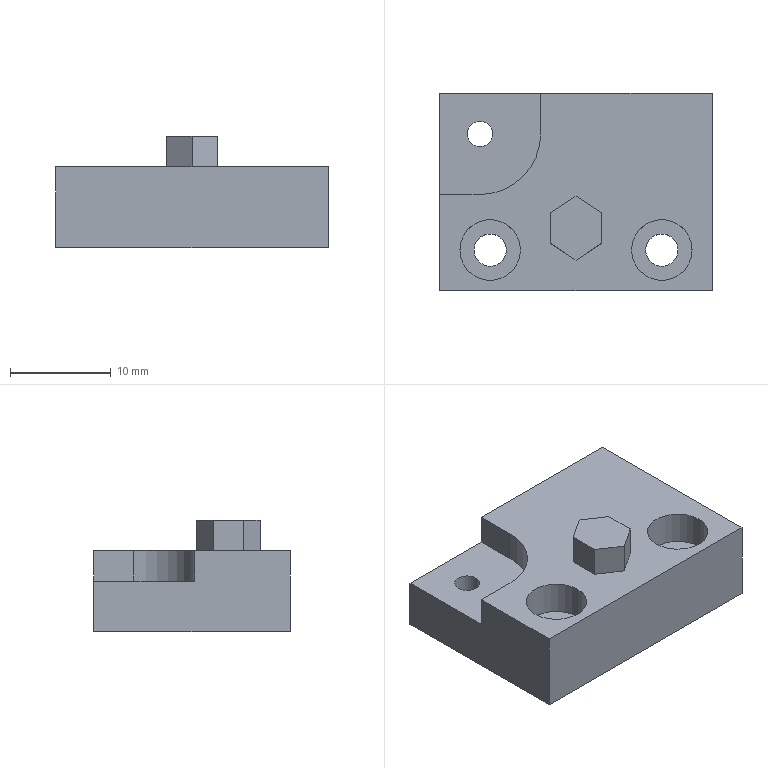Part | NX | 1 solid | 33 faces | box 27 x 19.5 x 11 mm | volume 3538 mm3 | plane 18 | cylinder 13 | cone 2 | commonest cylinder face diameters 3.2 x4 6 x4 2.5 x2 4.2 x2 12 x1
STEP:
#1=CARTESIAN_POINT('',(27.,0.,0.));
#2=VERTEX_POINT('',#1);
#3=CARTESIAN_POINT('',(0.,0.,0.));
#4=VERTEX_POINT('',#3);
#5=CARTESIAN_POINT('',(27.,0.,0.));
#6=DIRECTION('',(-1.,0.,0.));
#7=VECTOR('',#6,1000.);
#8=LINE('',#5,#7);
#9=EDGE_CURVE('',#2,#4,#8,.T.);
#10=ORIENTED_EDGE('',*,*,#9,.T.);
#11=CARTESIAN_POINT('',(0.,19.5,0.));
#12=VERTEX_POINT('',#11);
#13=CARTESIAN_POINT('',(0.,0.,0.));
#14=DIRECTION('',(0.,1.,0.));
#15=VECTOR('',#14,1000.);
#16=LINE('',#13,#15);
#17=EDGE_CURVE('',#4,#12,#16,.T.);
#18=ORIENTED_EDGE('',*,*,#17,.T.);
#19=CARTESIAN_POINT('',(27.,19.5,0.));
#20=VERTEX_POINT('',#19);
#21=CARTESIAN_POINT('',(0.,19.5,0.));
#22=DIRECTION('',(1.,0.,0.));
#23=VECTOR('',#22,1000.);
#24=LINE('',#21,#23);
#25=EDGE_CURVE('',#12,#20,#24,.T.);
#26=ORIENTED_EDGE('',*,*,#25,.T.);
#27=CARTESIAN_POINT('',(27.,19.5,0.));
#28=DIRECTION('',(0.,-1.,0.));
#29=VECTOR('',#28,1000.);
#30=LINE('',#27,#29);
#31=EDGE_CURVE('',#20,#2,#30,.T.);
#32=ORIENTED_EDGE('',*,*,#31,.T.);
#33=EDGE_LOOP('',(#10,#18,#26,#32));
#34=FACE_BOUND('',#33,.T.);
#35=CARTESIAN_POINT('',(6.6,4.,0.));
#36=VERTEX_POINT('',#35);
#37=CARTESIAN_POINT('',(3.4,4.,0.));
#38=VERTEX_POINT('',#37);
#39=CARTESIAN_POINT('',(5.,4.,0.));
#40=DIRECTION('',(0.,0.,-1.));
#41=DIRECTION('',(-1.,0.,0.));
#42=AXIS2_PLACEMENT_3D('',#39,#40,#41);
#43=CIRCLE('',#42,1.6);
#44=EDGE_CURVE('',#36,#38,#43,.T.);
#45=ORIENTED_EDGE('',*,*,#44,.F.);
#46=CARTESIAN_POINT('',(5.,4.,0.));
#47=DIRECTION('',(0.,0.,-1.));
#48=DIRECTION('',(-1.,0.,0.));
#49=AXIS2_PLACEMENT_3D('',#46,#47,#48);
#50=CIRCLE('',#49,1.6);
#51=EDGE_CURVE('',#38,#36,#50,.T.);
#52=ORIENTED_EDGE('',*,*,#51,.F.);
#53=EDGE_LOOP('',(#45,#52));
#54=FACE_BOUND('',#53,.T.);
#55=CARTESIAN_POINT('',(20.4,4.,0.));
#56=VERTEX_POINT('',#55);
#57=CARTESIAN_POINT('',(23.6,4.,0.));
#58=VERTEX_POINT('',#57);
#59=CARTESIAN_POINT('',(22.,4.,0.));
#60=DIRECTION('',(0.,0.,-1.));
#61=DIRECTION('',(-1.,0.,0.));
#62=AXIS2_PLACEMENT_3D('',#59,#60,#61);
#63=CIRCLE('',#62,1.6);
#64=EDGE_CURVE('',#56,#58,#63,.T.);
#65=ORIENTED_EDGE('',*,*,#64,.F.);
#66=CARTESIAN_POINT('',(22.,4.,0.));
#67=DIRECTION('',(0.,0.,-1.));
#68=DIRECTION('',(-1.,0.,0.));
#69=AXIS2_PLACEMENT_3D('',#66,#67,#68);
#70=CIRCLE('',#69,1.6);
#71=EDGE_CURVE('',#58,#56,#70,.T.);
#72=ORIENTED_EDGE('',*,*,#71,.F.);
#73=EDGE_LOOP('',(#65,#72));
#74=FACE_BOUND('',#73,.T.);
#75=CARTESIAN_POINT('',(2.75,15.5,0.));
#76=VERTEX_POINT('',#75);
#77=CARTESIAN_POINT('',(5.25,15.5,0.));
#78=VERTEX_POINT('',#77);
#79=CARTESIAN_POINT('',(4.,15.5,0.));
#80=DIRECTION('',(0.,0.,-1.));
#81=DIRECTION('',(-1.,0.,0.));
#82=AXIS2_PLACEMENT_3D('',#79,#80,#81);
#83=CIRCLE('',#82,1.25);
#84=EDGE_CURVE('',#76,#78,#83,.T.);
#85=ORIENTED_EDGE('',*,*,#84,.F.);
#86=CARTESIAN_POINT('',(4.,15.5,0.));
#87=DIRECTION('',(0.,0.,-1.));
#88=DIRECTION('',(-1.,0.,0.));
#89=AXIS2_PLACEMENT_3D('',#86,#87,#88);
#90=CIRCLE('',#89,1.25);
#91=EDGE_CURVE('',#78,#76,#90,.T.);
#92=ORIENTED_EDGE('',*,*,#91,.F.);
#93=EDGE_LOOP('',(#85,#92));
#94=FACE_BOUND('',#93,.T.);
#95=CARTESIAN_POINT('',(0.,0.,0.));
#96=DIRECTION('',(0.,0.,1.));
#97=DIRECTION('',(1.,0.,0.));
#98=AXIS2_PLACEMENT_3D('',#95,#96,#97);
#99=PLANE('',#98);
#100=ADVANCED_FACE('',(#34,#54,#74,#94),#99,.F.);
#101=ORIENTED_EDGE('',*,*,#9,.F.);
#102=CARTESIAN_POINT('',(27.,0.,8.));
#103=VERTEX_POINT('',#102);
#104=CARTESIAN_POINT('',(27.,0.,8.));
#105=DIRECTION('',(0.,0.,-1.));
#106=VECTOR('',#105,1000.);
#107=LINE('',#104,#106);
#108=EDGE_CURVE('',#103,#2,#107,.T.);
#109=ORIENTED_EDGE('',*,*,#108,.F.);
#110=CARTESIAN_POINT('',(0.,0.,8.));
#111=VERTEX_POINT('',#110);
#112=CARTESIAN_POINT('',(27.,0.,8.));
#113=DIRECTION('',(-1.,0.,0.));
#114=VECTOR('',#113,1000.);
#115=LINE('',#112,#114);
#116=EDGE_CURVE('',#103,#111,#115,.T.);
#117=ORIENTED_EDGE('',*,*,#116,.T.);
#118=CARTESIAN_POINT('',(0.,0.,8.));
#119=DIRECTION('',(0.,0.,-1.));
#120=VECTOR('',#119,1000.);
#121=LINE('',#118,#120);
#122=EDGE_CURVE('',#111,#4,#121,.T.);
#123=ORIENTED_EDGE('',*,*,#122,.T.);
#124=EDGE_LOOP('',(#101,#109,#117,#123));
#125=FACE_BOUND('',#124,.T.);
#126=CARTESIAN_POINT('',(0.,0.,0.));
#127=DIRECTION('',(0.,-1.,0.));
#128=DIRECTION('',(0.,0.,-1.));
#129=AXIS2_PLACEMENT_3D('',#126,#127,#128);
#130=PLANE('',#129);
#131=ADVANCED_FACE('',(#125),#130,.T.);
#132=CARTESIAN_POINT('',(0.,9.5,5.));
#133=VERTEX_POINT('',#132);
#134=CARTESIAN_POINT('',(0.,9.5,8.));
#135=VERTEX_POINT('',#134);
#136=CARTESIAN_POINT('',(0.,9.5,5.));
#137=DIRECTION('',(0.,0.,1.));
#138=VECTOR('',#137,1000.);
#139=LINE('',#136,#138);
#140=EDGE_CURVE('',#133,#135,#139,.T.);
#141=ORIENTED_EDGE('',*,*,#140,.F.);
#142=CARTESIAN_POINT('',(0.,19.5,5.));
#143=VERTEX_POINT('',#142);
#144=CARTESIAN_POINT('',(0.,9.5,5.));
#145=DIRECTION('',(0.,1.,0.));
#146=VECTOR('',#145,1000.);
#147=LINE('',#144,#146);
#148=EDGE_CURVE('',#133,#143,#147,.T.);
#149=ORIENTED_EDGE('',*,*,#148,.T.);
#150=CARTESIAN_POINT('',(0.,19.5,5.));
#151=DIRECTION('',(0.,0.,-1.));
#152=VECTOR('',#151,1000.);
#153=LINE('',#150,#152);
#154=EDGE_CURVE('',#143,#12,#153,.T.);
#155=ORIENTED_EDGE('',*,*,#154,.T.);
#156=ORIENTED_EDGE('',*,*,#17,.F.);
#157=ORIENTED_EDGE('',*,*,#122,.F.);
#158=CARTESIAN_POINT('',(0.,0.,8.));
#159=DIRECTION('',(0.,1.,0.));
#160=VECTOR('',#159,1000.);
#161=LINE('',#158,#160);
#162=EDGE_CURVE('',#111,#135,#161,.T.);
#163=ORIENTED_EDGE('',*,*,#162,.T.);
#164=EDGE_LOOP('',(#141,#149,#155,#156,#157,#163));
#165=FACE_BOUND('',#164,.T.);
#166=CARTESIAN_POINT('',(0.,19.5,0.));
#167=DIRECTION('',(-1.,0.,0.));
#168=DIRECTION('',(0.,0.,1.));
#169=AXIS2_PLACEMENT_3D('',#166,#167,#168);
#170=PLANE('',#169);
#171=ADVANCED_FACE('',(#165),#170,.T.);
#172=CARTESIAN_POINT('',(4.,9.5,8.));
#173=VERTEX_POINT('',#172);
#174=CARTESIAN_POINT('',(4.,9.5,8.));
#175=DIRECTION('',(-1.,0.,0.));
#176=VECTOR('',#175,1000.);
#177=LINE('',#174,#176);
#178=EDGE_CURVE('',#173,#135,#177,.T.);
#179=ORIENTED_EDGE('',*,*,#178,.F.);
#180=CARTESIAN_POINT('',(4.,9.5,5.));
#181=VERTEX_POINT('',#180);
#182=CARTESIAN_POINT('',(4.,9.5,8.));
#183=DIRECTION('',(0.,0.,-1.));
#184=VECTOR('',#183,1000.);
#185=LINE('',#182,#184);
#186=EDGE_CURVE('',#173,#181,#185,.T.);
#187=ORIENTED_EDGE('',*,*,#186,.T.);
#188=CARTESIAN_POINT('',(4.,9.5,5.));
#189=DIRECTION('',(-1.,0.,0.));
#190=VECTOR('',#189,1000.);
#191=LINE('',#188,#190);
#192=EDGE_CURVE('',#181,#133,#191,.T.);
#193=ORIENTED_EDGE('',*,*,#192,.T.);
#194=ORIENTED_EDGE('',*,*,#140,.T.);
#195=EDGE_LOOP('',(#179,#187,#193,#194));
#196=FACE_BOUND('',#195,.T.);
#197=CARTESIAN_POINT('',(0.,9.5,8.));
#198=DIRECTION('',(0.,-1.,0.));
#199=DIRECTION('',(0.,0.,-1.));
#200=AXIS2_PLACEMENT_3D('',#197,#198,#199);
#201=PLANE('',#200);
#202=ADVANCED_FACE('',(#196),#201,.F.);
#203=ORIENTED_EDGE('',*,*,#178,.T.);
#204=ORIENTED_EDGE('',*,*,#162,.F.);
#205=ORIENTED_EDGE('',*,*,#116,.F.);
#206=CARTESIAN_POINT('',(27.,19.5,8.));
#207=VERTEX_POINT('',#206);
#208=CARTESIAN_POINT('',(27.,19.5,8.));
#209=DIRECTION('',(0.,-1.,0.));
#210=VECTOR('',#209,1000.);
#211=LINE('',#208,#210);
#212=EDGE_CURVE('',#207,#103,#211,.T.);
#213=ORIENTED_EDGE('',*,*,#212,.F.);
#214=CARTESIAN_POINT('',(10.,19.5,8.));
#215=VERTEX_POINT('',#214);
#216=CARTESIAN_POINT('',(10.,19.5,8.));
#217=DIRECTION('',(1.,0.,0.));
#218=VECTOR('',#217,1000.);
#219=LINE('',#216,#218);
#220=EDGE_CURVE('',#215,#207,#219,.T.);
#221=ORIENTED_EDGE('',*,*,#220,.F.);
#222=CARTESIAN_POINT('',(10.,15.5,8.));
#223=VERTEX_POINT('',#222);
#224=CARTESIAN_POINT('',(10.,15.5,8.));
#225=DIRECTION('',(0.,1.,0.));
#226=VECTOR('',#225,1000.);
#227=LINE('',#224,#226);
#228=EDGE_CURVE('',#223,#215,#227,.T.);
#229=ORIENTED_EDGE('',*,*,#228,.F.);
#230=CARTESIAN_POINT('',(4.,15.5,8.));
#231=DIRECTION('',(0.,0.,1.));
#232=DIRECTION('',(0.,-1.,0.));
#233=AXIS2_PLACEMENT_3D('',#230,#231,#232);
#234=CIRCLE('',#233,6.);
#235=EDGE_CURVE('',#173,#223,#234,.T.);
#236=ORIENTED_EDGE('',*,*,#235,.F.);
#237=EDGE_LOOP('',(#203,#204,#205,#213,#221,#229,#236));
#238=FACE_BOUND('',#237,.T.);
#239=CARTESIAN_POINT('',(8.,4.,8.));
#240=VERTEX_POINT('',#239);
#241=CARTESIAN_POINT('',(2.,4.,8.));
#242=VERTEX_POINT('',#241);
#243=CARTESIAN_POINT('',(5.,4.,8.));
#244=DIRECTION('',(0.,0.,1.));
#245=DIRECTION('',(1.,0.,0.));
#246=AXIS2_PLACEMENT_3D('',#243,#244,#245);
#247=CIRCLE('',#246,3.);
#248=EDGE_CURVE('',#240,#242,#247,.T.);
#249=ORIENTED_EDGE('',*,*,#248,.F.);
#250=CARTESIAN_POINT('',(5.,4.,8.));
#251=DIRECTION('',(0.,0.,1.));
#252=DIRECTION('',(1.,0.,0.));
#253=AXIS2_PLACEMENT_3D('',#250,#251,#252);
#254=CIRCLE('',#253,3.);
#255=EDGE_CURVE('',#242,#240,#254,.T.);
#256=ORIENTED_EDGE('',*,*,#255,.F.);
#257=EDGE_LOOP('',(#249,#256));
#258=FACE_BOUND('',#257,.T.);
#259=CARTESIAN_POINT('',(19.,4.,8.));
#260=VERTEX_POINT('',#259);
#261=CARTESIAN_POINT('',(25.,4.,8.));
#262=VERTEX_POINT('',#261);
#263=CARTESIAN_POINT('',(22.,4.,8.));
#264=DIRECTION('',(0.,0.,1.));
#265=DIRECTION('',(1.,0.,0.));
#266=AXIS2_PLACEMENT_3D('',#263,#264,#265);
#267=CIRCLE('',#266,3.);
#268=EDGE_CURVE('',#260,#262,#267,.T.);
#269=ORIENTED_EDGE('',*,*,#268,.F.);
#270=CARTESIAN_POINT('',(22.,4.,8.));
#271=DIRECTION('',(0.,0.,1.));
#272=DIRECTION('',(1.,0.,0.));
#273=AXIS2_PLACEMENT_3D('',#270,#271,#272);
#274=CIRCLE('',#273,3.);
#275=EDGE_CURVE('',#262,#260,#274,.T.);
#276=ORIENTED_EDGE('',*,*,#275,.F.);
#277=EDGE_LOOP('',(#269,#276));
#278=FACE_BOUND('',#277,.T.);
#279=CARTESIAN_POINT('',(13.5,9.317,8.));
#280=VERTEX_POINT('',#279);
#281=CARTESIAN_POINT('',(11.,7.658,8.));
#282=VERTEX_POINT('',#281);
#283=CARTESIAN_POINT('',(13.5,9.317,8.));
#284=DIRECTION('',(-0.8333,-0.5528,0.));
#285=VECTOR('',#284,1000.);
#286=LINE('',#283,#285);
#287=EDGE_CURVE('',#280,#282,#286,.T.);
#288=ORIENTED_EDGE('',*,*,#287,.F.);
#289=CARTESIAN_POINT('',(16.,7.658,8.));
#290=VERTEX_POINT('',#289);
#291=CARTESIAN_POINT('',(16.,7.658,8.));
#292=DIRECTION('',(-0.8333,0.5528,0.));
#293=VECTOR('',#292,1000.);
#294=LINE('',#291,#293);
#295=EDGE_CURVE('',#290,#280,#294,.T.);
#296=ORIENTED_EDGE('',*,*,#295,.F.);
#297=CARTESIAN_POINT('',(16.,4.658,8.));
#298=VERTEX_POINT('',#297);
#299=CARTESIAN_POINT('',(16.,7.658,8.));
#300=DIRECTION('',(0.,-1.,0.));
#301=VECTOR('',#300,1000.);
#302=LINE('',#299,#301);
#303=EDGE_CURVE('',#290,#298,#302,.T.);
#304=ORIENTED_EDGE('',*,*,#303,.T.);
#305=CARTESIAN_POINT('',(13.5,3.,8.));
#306=VERTEX_POINT('',#305);
#307=CARTESIAN_POINT('',(13.5,3.,8.));
#308=DIRECTION('',(0.8333,0.5528,0.));
#309=VECTOR('',#308,1000.);
#310=LINE('',#307,#309);
#311=EDGE_CURVE('',#306,#298,#310,.T.);
#312=ORIENTED_EDGE('',*,*,#311,.F.);
#313=CARTESIAN_POINT('',(11.,4.658,8.));
#314=VERTEX_POINT('',#313);
#315=CARTESIAN_POINT('',(11.,4.658,8.));
#316=DIRECTION('',(0.8333,-0.5528,0.));
#317=VECTOR('',#316,1000.);
#318=LINE('',#315,#317);
#319=EDGE_CURVE('',#314,#306,#318,.T.);
#320=ORIENTED_EDGE('',*,*,#319,.F.);
#321=CARTESIAN_POINT('',(11.,4.658,8.));
#322=DIRECTION('',(0.,1.,0.));
#323=VECTOR('',#322,1000.);
#324=LINE('',#321,#323);
#325=EDGE_CURVE('',#314,#282,#324,.T.);
#326=ORIENTED_EDGE('',*,*,#325,.T.);
#327=EDGE_LOOP('',(#288,#296,#304,#312,#320,#326));
#328=FACE_BOUND('',#327,.T.);
#329=CARTESIAN_POINT('',(0.,0.,8.));
#330=DIRECTION('',(0.,0.,1.));
#331=DIRECTION('',(1.,0.,0.));
#332=AXIS2_PLACEMENT_3D('',#329,#330,#331);
#333=PLANE('',#332);
#334=ADVANCED_FACE('',(#238,#258,#278,#328),#333,.T.);
#335=ORIENTED_EDGE('',*,*,#235,.T.);
#336=CARTESIAN_POINT('',(10.,15.5,5.));
#337=VERTEX_POINT('',#336);
#338=CARTESIAN_POINT('',(10.,15.5,8.));
#339=DIRECTION('',(0.,0.,1.));
#340=VECTOR('',#339,1000.);
#341=LINE('',#338,#340);
#342=EDGE_CURVE('',#337,#223,#341,.T.);
#343=ORIENTED_EDGE('',*,*,#342,.F.);
#344=CARTESIAN_POINT('',(4.,15.5,5.));
#345=DIRECTION('',(0.,0.,-1.));
#346=DIRECTION('',(1.,0.,0.));
#347=AXIS2_PLACEMENT_3D('',#344,#345,#346);
#348=CIRCLE('',#347,6.);
#349=EDGE_CURVE('',#337,#181,#348,.T.);
#350=ORIENTED_EDGE('',*,*,#349,.T.);
#351=ORIENTED_EDGE('',*,*,#186,.F.);
#352=EDGE_LOOP('',(#335,#343,#350,#351));
#353=FACE_BOUND('',#352,.T.);
#354=CARTESIAN_POINT('',(4.,15.5,8.));
#355=DIRECTION('',(0.,0.,1.));
#356=DIRECTION('',(1.,0.,0.));
#357=AXIS2_PLACEMENT_3D('',#354,#355,#356);
#358=CYLINDRICAL_SURFACE('',#357,6.);
#359=ADVANCED_FACE('',(#353),#358,.F.);
#360=ORIENTED_EDGE('',*,*,#148,.F.);
#361=ORIENTED_EDGE('',*,*,#192,.F.);
#362=ORIENTED_EDGE('',*,*,#349,.F.);
#363=CARTESIAN_POINT('',(10.,19.5,5.));
#364=VERTEX_POINT('',#363);
#365=CARTESIAN_POINT('',(10.,19.5,5.));
#366=DIRECTION('',(0.,-1.,0.));
#367=VECTOR('',#366,1000.);
#368=LINE('',#365,#367);
#369=EDGE_CURVE('',#364,#337,#368,.T.);
#370=ORIENTED_EDGE('',*,*,#369,.F.);
#371=CARTESIAN_POINT('',(0.,19.5,5.));
#372=DIRECTION('',(1.,0.,0.));
#373=VECTOR('',#372,1000.);
#374=LINE('',#371,#373);
#375=EDGE_CURVE('',#143,#364,#374,.T.);
#376=ORIENTED_EDGE('',*,*,#375,.F.);
#377=EDGE_LOOP('',(#360,#361,#362,#370,#376));
#378=FACE_BOUND('',#377,.T.);
#379=CARTESIAN_POINT('',(5.25,15.5,5.));
#380=VERTEX_POINT('',#379);
#381=CARTESIAN_POINT('',(2.75,15.5,5.));
#382=VERTEX_POINT('',#381);
#383=CARTESIAN_POINT('',(4.,15.5,5.));
#384=DIRECTION('',(0.,0.,1.));
#385=DIRECTION('',(1.,0.,0.));
#386=AXIS2_PLACEMENT_3D('',#383,#384,#385);
#387=CIRCLE('',#386,1.25);
#388=EDGE_CURVE('',#380,#382,#387,.T.);
#389=ORIENTED_EDGE('',*,*,#388,.F.);
#390=CARTESIAN_POINT('',(4.,15.5,5.));
#391=DIRECTION('',(0.,0.,1.));
#392=DIRECTION('',(1.,0.,0.));
#393=AXIS2_PLACEMENT_3D('',#390,#391,#392);
#394=CIRCLE('',#393,1.25);
#395=EDGE_CURVE('',#382,#380,#394,.T.);
#396=ORIENTED_EDGE('',*,*,#395,.F.);
#397=EDGE_LOOP('',(#389,#396));
#398=FACE_BOUND('',#397,.T.);
#399=CARTESIAN_POINT('',(0.,0.,5.));
#400=DIRECTION('',(0.,0.,1.));
#401=DIRECTION('',(1.,0.,0.));
#402=AXIS2_PLACEMENT_3D('',#399,#400,#401);
#403=PLANE('',#402);
#404=ADVANCED_FACE('',(#378,#398),#403,.T.);
#405=CARTESIAN_POINT('',(10.,19.5,5.));
#406=DIRECTION('',(0.,0.,1.));
#407=VECTOR('',#406,1000.);
#408=LINE('',#405,#407);
#409=EDGE_CURVE('',#364,#215,#408,.T.);
#410=ORIENTED_EDGE('',*,*,#409,.T.);
#411=ORIENTED_EDGE('',*,*,#220,.T.);
#412=CARTESIAN_POINT('',(27.,19.5,8.));
#413=DIRECTION('',(0.,0.,-1.));
#414=VECTOR('',#413,1000.);
#415=LINE('',#412,#414);
#416=EDGE_CURVE('',#207,#20,#415,.T.);
#417=ORIENTED_EDGE('',*,*,#416,.T.);
#418=ORIENTED_EDGE('',*,*,#25,.F.);
#419=ORIENTED_EDGE('',*,*,#154,.F.);
#420=ORIENTED_EDGE('',*,*,#375,.T.);
#421=EDGE_LOOP('',(#410,#411,#417,#418,#419,#420));
#422=FACE_BOUND('',#421,.T.);
#423=CARTESIAN_POINT('',(27.,19.5,0.));
#424=DIRECTION('',(0.,1.,0.));
#425=DIRECTION('',(1.,0.,0.));
#426=AXIS2_PLACEMENT_3D('',#423,#424,#425);
#427=PLANE('',#426);
#428=ADVANCED_FACE('',(#422),#427,.T.);
#429=ORIENTED_EDGE('',*,*,#228,.T.);
#430=ORIENTED_EDGE('',*,*,#409,.F.);
#431=ORIENTED_EDGE('',*,*,#369,.T.);
#432=ORIENTED_EDGE('',*,*,#342,.T.);
#433=EDGE_LOOP('',(#429,#430,#431,#432));
#434=FACE_BOUND('',#433,.T.);
#435=CARTESIAN_POINT('',(10.,15.5,8.));
#436=DIRECTION('',(1.,0.,0.));
#437=DIRECTION('',(0.,1.,0.));
#438=AXIS2_PLACEMENT_3D('',#435,#436,#437);
#439=PLANE('',#438);
#440=ADVANCED_FACE('',(#434),#439,.F.);
#441=ORIENTED_EDGE('',*,*,#31,.F.);
#442=ORIENTED_EDGE('',*,*,#416,.F.);
#443=ORIENTED_EDGE('',*,*,#212,.T.);
#444=ORIENTED_EDGE('',*,*,#108,.T.);
#445=EDGE_LOOP('',(#441,#442,#443,#444));
#446=FACE_BOUND('',#445,.T.);
#447=CARTESIAN_POINT('',(27.,12.1,4.));
#448=VERTEX_POINT('',#447);
#449=CARTESIAN_POINT('',(27.,7.9,4.));
#450=VERTEX_POINT('',#449);
#451=CARTESIAN_POINT('',(27.,10.,4.));
#452=DIRECTION('',(1.,0.,0.));
#453=DIRECTION('',(0.,1.,0.));
#454=AXIS2_PLACEMENT_3D('',#451,#452,#453);
#455=CIRCLE('',#454,2.1);
#456=EDGE_CURVE('',#448,#450,#455,.T.);
#457=ORIENTED_EDGE('',*,*,#456,.F.);
#458=CARTESIAN_POINT('',(27.,10.,4.));
#459=DIRECTION('',(1.,0.,0.));
#460=DIRECTION('',(0.,1.,0.));
#461=AXIS2_PLACEMENT_3D('',#458,#459,#460);
#462=CIRCLE('',#461,2.1);
#463=EDGE_CURVE('',#450,#448,#462,.T.);
#464=ORIENTED_EDGE('',*,*,#463,.F.);
#465=EDGE_LOOP('',(#457,#464));
#466=FACE_BOUND('',#465,.T.);
#467=CARTESIAN_POINT('',(27.,0.,0.));
#468=DIRECTION('',(1.,0.,0.));
#469=DIRECTION('',(0.,1.,0.));
#470=AXIS2_PLACEMENT_3D('',#467,#468,#469);
#471=PLANE('',#470);
#472=ADVANCED_FACE('',(#446,#466),#471,.T.);
#473=CARTESIAN_POINT('',(14.4,12.1,4.));
#474=VERTEX_POINT('',#473);
#475=CARTESIAN_POINT('',(14.4,7.9,4.));
#476=VERTEX_POINT('',#475);
#477=CARTESIAN_POINT('',(14.4,10.,4.));
#478=DIRECTION('',(-1.,0.,0.));
#479=DIRECTION('',(0.,-1.,0.));
#480=AXIS2_PLACEMENT_3D('',#477,#478,#479);
#481=CIRCLE('',#480,2.1);
#482=EDGE_CURVE('',#474,#476,#481,.T.);
#483=ORIENTED_EDGE('',*,*,#482,.T.);
#484=CARTESIAN_POINT('',(12.445,7.9,4.));
#485=DIRECTION('',(1.,0.,0.));
#486=VECTOR('',#485,1000.);
#487=LINE('',#484,#486);
#488=EDGE_CURVE('',#450,#476,#487,.F.);
#489=ORIENTED_EDGE('',*,*,#488,.F.);
#490=ORIENTED_EDGE('',*,*,#463,.T.);
#491=CARTESIAN_POINT('',(12.445,12.1,4.));
#492=DIRECTION('',(1.,0.,0.));
#493=VECTOR('',#492,1000.);
#494=LINE('',#491,#493);
#495=EDGE_CURVE('',#448,#474,#494,.F.);
#496=ORIENTED_EDGE('',*,*,#495,.T.);
#497=EDGE_LOOP('',(#483,#489,#490,#496));
#498=FACE_BOUND('',#497,.T.);
#499=CARTESIAN_POINT('',(12.445,10.,4.));
#500=DIRECTION('',(1.,0.,0.));
#501=DIRECTION('',(0.,-1.,0.));
#502=AXIS2_PLACEMENT_3D('',#499,#500,#501);
#503=CYLINDRICAL_SURFACE('',#502,2.1);
#504=ADVANCED_FACE('',(#498),#503,.F.);
#505=ORIENTED_EDGE('',*,*,#325,.F.);
#506=CARTESIAN_POINT('',(11.,4.658,11.));
#507=VERTEX_POINT('',#506);
#508=CARTESIAN_POINT('',(11.,4.658,11.));
#509=DIRECTION('',(0.,0.,-1.));
#510=VECTOR('',#509,1000.);
#511=LINE('',#508,#510);
#512=EDGE_CURVE('',#507,#314,#511,.T.);
#513=ORIENTED_EDGE('',*,*,#512,.F.);
#514=CARTESIAN_POINT('',(11.,7.658,11.));
#515=VERTEX_POINT('',#514);
#516=CARTESIAN_POINT('',(11.,4.658,11.));
#517=DIRECTION('',(0.,1.,0.));
#518=VECTOR('',#517,1000.);
#519=LINE('',#516,#518);
#520=EDGE_CURVE('',#507,#515,#519,.T.);
#521=ORIENTED_EDGE('',*,*,#520,.T.);
#522=CARTESIAN_POINT('',(11.,7.658,11.));
#523=DIRECTION('',(0.,0.,-1.));
#524=VECTOR('',#523,1000.);
#525=LINE('',#522,#524);
#526=EDGE_CURVE('',#515,#282,#525,.T.);
#527=ORIENTED_EDGE('',*,*,#526,.T.);
#528=EDGE_LOOP('',(#505,#513,#521,#527));
#529=FACE_BOUND('',#528,.T.);
#530=CARTESIAN_POINT('',(11.,7.658,8.));
#531=DIRECTION('',(-1.,0.,0.));
#532=DIRECTION('',(0.,0.,1.));
#533=AXIS2_PLACEMENT_3D('',#530,#531,#532);
#534=PLANE('',#533);
#535=ADVANCED_FACE('',(#529),#534,.T.);
#536=CARTESIAN_POINT('',(13.138,10.,4.));
#537=VERTEX_POINT('',#536);
#538=CARTESIAN_POINT('',(13.782,11.071,4.));
#539=DIRECTION('',(0.515,0.8572,0.));
#540=VECTOR('',#539,1000.);
#541=LINE('',#538,#540);
#542=EDGE_CURVE('',#537,#474,#541,.T.);
#543=ORIENTED_EDGE('',*,*,#542,.T.);
#544=CARTESIAN_POINT('',(14.4,10.,4.));
#545=DIRECTION('',(-1.,0.,0.));
#546=DIRECTION('',(0.,-1.,0.));
#547=AXIS2_PLACEMENT_3D('',#544,#545,#546);
#548=CIRCLE('',#547,2.1);
#549=EDGE_CURVE('',#476,#474,#548,.T.);
#550=ORIENTED_EDGE('',*,*,#549,.F.);
#551=CARTESIAN_POINT('',(13.782,8.929,4.));
#552=DIRECTION('',(0.515,-0.8572,0.));
#553=VECTOR('',#552,1000.);
#554=LINE('',#551,#553);
#555=EDGE_CURVE('',#537,#476,#554,.T.);
#556=ORIENTED_EDGE('',*,*,#555,.F.);
#557=EDGE_LOOP('',(#543,#550,#556));
#558=FACE_BOUND('',#557,.T.);
#559=CARTESIAN_POINT('',(13.782,10.,4.));
#560=DIRECTION('',(1.,0.,0.));
#561=DIRECTION('',(0.,-1.,0.));
#562=AXIS2_PLACEMENT_3D('',#559,#560,#561);
#563=CONICAL_SURFACE('',#562,1.071,1.03);
#564=ADVANCED_FACE('',(#558),#563,.F.);
#565=CARTESIAN_POINT('',(13.5,9.317,11.));
#566=VERTEX_POINT('',#565);
#567=CARTESIAN_POINT('',(11.,7.658,11.));
#568=DIRECTION('',(0.8333,0.5528,0.));
#569=VECTOR('',#568,1000.);
#570=LINE('',#567,#569);
#571=EDGE_CURVE('',#515,#566,#570,.T.);
#572=ORIENTED_EDGE('',*,*,#571,.F.);
#573=ORIENTED_EDGE('',*,*,#520,.F.);
#574=CARTESIAN_POINT('',(13.5,3.,11.));
#575=VERTEX_POINT('',#574);
#576=CARTESIAN_POINT('',(13.5,3.,11.));
#577=DIRECTION('',(-0.8333,0.5528,0.));
#578=VECTOR('',#577,1000.);
#579=LINE('',#576,#578);
#580=EDGE_CURVE('',#575,#507,#579,.T.);
#581=ORIENTED_EDGE('',*,*,#580,.F.);
#582=CARTESIAN_POINT('',(16.,4.658,11.));
#583=VERTEX_POINT('',#582);
#584=CARTESIAN_POINT('',(16.,4.658,11.));
#585=DIRECTION('',(-0.8333,-0.5528,0.));
#586=VECTOR('',#585,1000.);
#587=LINE('',#584,#586);
#588=EDGE_CURVE('',#583,#575,#587,.T.);
#589=ORIENTED_EDGE('',*,*,#588,.F.);
#590=CARTESIAN_POINT('',(16.,7.658,11.));
#591=VERTEX_POINT('',#590);
#592=CARTESIAN_POINT('',(16.,7.658,11.));
#593=DIRECTION('',(0.,-1.,0.));
#594=VECTOR('',#593,1000.);
#595=LINE('',#592,#594);
#596=EDGE_CURVE('',#591,#583,#595,.T.);
#597=ORIENTED_EDGE('',*,*,#596,.F.);
#598=CARTESIAN_POINT('',(13.5,9.317,11.));
#599=DIRECTION('',(0.8333,-0.5528,0.));
#600=VECTOR('',#599,1000.);
#601=LINE('',#598,#600);
#602=EDGE_CURVE('',#566,#591,#601,.T.);
#603=ORIENTED_EDGE('',*,*,#602,.F.);
#604=EDGE_LOOP('',(#572,#573,#581,#589,#597,#603));
#605=FACE_BOUND('',#604,.T.);
#606=CARTESIAN_POINT('',(0.,0.,11.));
#607=DIRECTION('',(0.,0.,1.));
#608=DIRECTION('',(1.,0.,0.));
#609=AXIS2_PLACEMENT_3D('',#606,#607,#608);
#610=PLANE('',#609);
#611=ADVANCED_FACE('',(#605),#610,.T.);
#612=ORIENTED_EDGE('',*,*,#84,.T.);
#613=CARTESIAN_POINT('',(5.25,15.5,-2.455));
#614=DIRECTION('',(0.,0.,1.));
#615=VECTOR('',#614,1000.);
#616=LINE('',#613,#615);
#617=EDGE_CURVE('',#380,#78,#616,.F.);
#618=ORIENTED_EDGE('',*,*,#617,.F.);
#619=ORIENTED_EDGE('',*,*,#388,.T.);
#620=CARTESIAN_POINT('',(2.75,15.5,-2.455));
#621=DIRECTION('',(0.,0.,1.));
#622=VECTOR('',#621,1000.);
#623=LINE('',#620,#622);
#624=EDGE_CURVE('',#382,#76,#623,.F.);
#625=ORIENTED_EDGE('',*,*,#624,.T.);
#626=EDGE_LOOP('',(#612,#618,#619,#625));
#627=FACE_BOUND('',#626,.T.);
#628=CARTESIAN_POINT('',(4.,15.5,-2.455));
#629=DIRECTION('',(0.,0.,1.));
#630=DIRECTION('',(-1.,0.,0.));
#631=AXIS2_PLACEMENT_3D('',#628,#629,#630);
#632=CYLINDRICAL_SURFACE('',#631,1.25);
#633=ADVANCED_FACE('',(#627),#632,.F.);
#634=ORIENTED_EDGE('',*,*,#287,.T.);
#635=ORIENTED_EDGE('',*,*,#526,.F.);
#636=ORIENTED_EDGE('',*,*,#571,.T.);
#637=CARTESIAN_POINT('',(13.5,9.317,11.));
#638=DIRECTION('',(0.,0.,-1.));
#639=VECTOR('',#638,1000.);
#640=LINE('',#637,#639);
#641=EDGE_CURVE('',#566,#280,#640,.T.);
#642=ORIENTED_EDGE('',*,*,#641,.T.);
#643=EDGE_LOOP('',(#634,#635,#636,#642));
#644=FACE_BOUND('',#643,.T.);
#645=CARTESIAN_POINT('',(13.5,9.317,8.));
#646=DIRECTION('',(-0.5528,0.8333,0.));
#647=DIRECTION('',(0.,0.,1.));
#648=AXIS2_PLACEMENT_3D('',#645,#646,#647);
#649=PLANE('',#648);
#650=ADVANCED_FACE('',(#644),#649,.T.);
#651=CARTESIAN_POINT('',(2.,4.,4.7));
#652=VERTEX_POINT('',#651);
#653=CARTESIAN_POINT('',(8.,4.,4.7));
#654=VERTEX_POINT('',#653);
#655=CARTESIAN_POINT('',(5.,4.,4.7));
#656=DIRECTION('',(0.,0.,-1.));
#657=DIRECTION('',(1.,0.,0.));
#658=AXIS2_PLACEMENT_3D('',#655,#656,#657);
#659=CIRCLE('',#658,3.);
#660=EDGE_CURVE('',#652,#654,#659,.T.);
#661=ORIENTED_EDGE('',*,*,#660,.T.);
#662=CARTESIAN_POINT('',(8.,4.,-1.24));
#663=DIRECTION('',(0.,0.,1.));
#664=VECTOR('',#663,1000.);
#665=LINE('',#662,#664);
#666=EDGE_CURVE('',#240,#654,#665,.F.);
#667=ORIENTED_EDGE('',*,*,#666,.F.);
#668=ORIENTED_EDGE('',*,*,#248,.T.);
#669=CARTESIAN_POINT('',(2.,4.,-1.24));
#670=DIRECTION('',(0.,0.,1.));
#671=VECTOR('',#670,1000.);
#672=LINE('',#669,#671);
#673=EDGE_CURVE('',#242,#652,#672,.F.);
#674=ORIENTED_EDGE('',*,*,#673,.T.);
#675=EDGE_LOOP('',(#661,#667,#668,#674));
#676=FACE_BOUND('',#675,.T.);
#677=CARTESIAN_POINT('',(5.,4.,-1.24));
#678=DIRECTION('',(0.,0.,1.));
#679=DIRECTION('',(-1.,0.,0.));
#680=AXIS2_PLACEMENT_3D('',#677,#678,#679);
#681=CYLINDRICAL_SURFACE('',#680,3.);
#682=ADVANCED_FACE('',(#676),#681,.F.);
#683=ORIENTED_EDGE('',*,*,#311,.T.);
#684=CARTESIAN_POINT('',(16.,4.658,11.));
#685=DIRECTION('',(0.,0.,-1.));
#686=VECTOR('',#685,1000.);
#687=LINE('',#684,#686);
#688=EDGE_CURVE('',#583,#298,#687,.T.);
#689=ORIENTED_EDGE('',*,*,#688,.F.);
#690=ORIENTED_EDGE('',*,*,#588,.T.);
#691=CARTESIAN_POINT('',(13.5,3.,11.));
#692=DIRECTION('',(0.,0.,-1.));
#693=VECTOR('',#692,1000.);
#694=LINE('',#691,#693);
#695=EDGE_CURVE('',#575,#306,#694,.T.);
#696=ORIENTED_EDGE('',*,*,#695,.T.);
#697=EDGE_LOOP('',(#683,#689,#690,#696));
#698=FACE_BOUND('',#697,.T.);
#699=CARTESIAN_POINT('',(13.5,3.,8.));
#700=DIRECTION('',(0.5528,-0.8333,0.));
#701=DIRECTION('',(0.,0.,-1.));
#702=AXIS2_PLACEMENT_3D('',#699,#700,#701);
#703=PLANE('',#702);
#704=ADVANCED_FACE('',(#698),#703,.T.);
#705=ORIENTED_EDGE('',*,*,#660,.F.);
#706=CARTESIAN_POINT('',(5.,4.,4.7));
#707=DIRECTION('',(0.,0.,-1.));
#708=DIRECTION('',(1.,0.,0.));
#709=AXIS2_PLACEMENT_3D('',#706,#707,#708);
#710=CIRCLE('',#709,3.);
#711=EDGE_CURVE('',#654,#652,#710,.T.);
#712=ORIENTED_EDGE('',*,*,#711,.F.);
#713=EDGE_LOOP('',(#705,#712));
#714=FACE_BOUND('',#713,.T.);
#715=CARTESIAN_POINT('',(6.6,4.,4.7));
#716=VERTEX_POINT('',#715);
#717=CARTESIAN_POINT('',(3.4,4.,4.7));
#718=VERTEX_POINT('',#717);
#719=CARTESIAN_POINT('',(5.,4.,4.7));
#720=DIRECTION('',(0.,0.,1.));
#721=DIRECTION('',(-1.,0.,0.));
#722=AXIS2_PLACEMENT_3D('',#719,#720,#721);
#723=CIRCLE('',#722,1.6);
#724=EDGE_CURVE('',#716,#718,#723,.T.);
#725=ORIENTED_EDGE('',*,*,#724,.F.);
#726=CARTESIAN_POINT('',(5.,4.,4.7));
#727=DIRECTION('',(0.,0.,1.));
#728=DIRECTION('',(-1.,0.,0.));
#729=AXIS2_PLACEMENT_3D('',#726,#727,#728);
#730=CIRCLE('',#729,1.6);
#731=EDGE_CURVE('',#718,#716,#730,.T.);
#732=ORIENTED_EDGE('',*,*,#731,.F.);
#733=EDGE_LOOP('',(#725,#732));
#734=FACE_BOUND('',#733,.T.);
#735=CARTESIAN_POINT('',(5.,4.,4.7));
#736=DIRECTION('',(0.,0.,1.));
#737=DIRECTION('',(1.,0.,0.));
#738=AXIS2_PLACEMENT_3D('',#735,#736,#737);
#739=PLANE('',#738);
#740=ADVANCED_FACE('',(#714,#734),#739,.T.);
#741=ORIENTED_EDGE('',*,*,#44,.T.);
#742=CARTESIAN_POINT('',(3.4,4.,-1.24));
#743=DIRECTION('',(0.,0.,1.));
#744=VECTOR('',#743,1000.);
#745=LINE('',#742,#744);
#746=EDGE_CURVE('',#718,#38,#745,.F.);
#747=ORIENTED_EDGE('',*,*,#746,.F.);
#748=ORIENTED_EDGE('',*,*,#731,.T.);
#749=CARTESIAN_POINT('',(6.6,4.,-1.24));
#750=DIRECTION('',(0.,0.,1.));
#751=VECTOR('',#750,1000.);
#752=LINE('',#749,#751);
#753=EDGE_CURVE('',#716,#36,#752,.F.);
#754=ORIENTED_EDGE('',*,*,#753,.T.);
#755=EDGE_LOOP('',(#741,#747,#748,#754));
#756=FACE_BOUND('',#755,.T.);
#757=CARTESIAN_POINT('',(5.,4.,-1.24));
#758=DIRECTION('',(0.,0.,1.));
#759=DIRECTION('',(-1.,0.,0.));
#760=AXIS2_PLACEMENT_3D('',#757,#758,#759);
#761=CYLINDRICAL_SURFACE('',#760,1.6);
#762=ADVANCED_FACE('',(#756),#761,.F.);
#763=ORIENTED_EDGE('',*,*,#295,.T.);
#764=ORIENTED_EDGE('',*,*,#641,.F.);
#765=ORIENTED_EDGE('',*,*,#602,.T.);
#766=CARTESIAN_POINT('',(16.,7.658,11.));
#767=DIRECTION('',(0.,0.,-1.));
#768=VECTOR('',#767,1000.);
#769=LINE('',#766,#768);
#770=EDGE_CURVE('',#591,#290,#769,.T.);
#771=ORIENTED_EDGE('',*,*,#770,.T.);
#772=EDGE_LOOP('',(#763,#764,#765,#771));
#773=FACE_BOUND('',#772,.T.);
#774=CARTESIAN_POINT('',(16.,7.658,8.));
#775=DIRECTION('',(0.5528,0.8333,0.));
#776=DIRECTION('',(0.,0.,-1.));
#777=AXIS2_PLACEMENT_3D('',#774,#775,#776);
#778=PLANE('',#777);
#779=ADVANCED_FACE('',(#773),#778,.T.);
#780=ORIENTED_EDGE('',*,*,#268,.T.);
#781=CARTESIAN_POINT('',(25.,4.,4.7));
#782=VERTEX_POINT('',#781);
#783=CARTESIAN_POINT('',(25.,4.,-1.24));
#784=DIRECTION('',(0.,0.,1.));
#785=VECTOR('',#784,1000.);
#786=LINE('',#783,#785);
#787=EDGE_CURVE('',#782,#262,#786,.T.);
#788=ORIENTED_EDGE('',*,*,#787,.F.);
#789=CARTESIAN_POINT('',(19.,4.,4.7));
#790=VERTEX_POINT('',#789);
#791=CARTESIAN_POINT('',(22.,4.,4.7));
#792=DIRECTION('',(0.,0.,-1.));
#793=DIRECTION('',(-1.,0.,0.));
#794=AXIS2_PLACEMENT_3D('',#791,#792,#793);
#795=CIRCLE('',#794,3.);
#796=EDGE_CURVE('',#782,#790,#795,.T.);
#797=ORIENTED_EDGE('',*,*,#796,.T.);
#798=CARTESIAN_POINT('',(19.,4.,-1.24));
#799=DIRECTION('',(0.,0.,1.));
#800=VECTOR('',#799,1000.);
#801=LINE('',#798,#800);
#802=EDGE_CURVE('',#790,#260,#801,.T.);
#803=ORIENTED_EDGE('',*,*,#802,.T.);
#804=EDGE_LOOP('',(#780,#788,#797,#803));
#805=FACE_BOUND('',#804,.T.);
#806=CARTESIAN_POINT('',(22.,4.,-1.24));
#807=DIRECTION('',(0.,0.,1.));
#808=DIRECTION('',(-1.,0.,0.));
#809=AXIS2_PLACEMENT_3D('',#806,#807,#808);
#810=CYLINDRICAL_SURFACE('',#809,3.);
#811=ADVANCED_FACE('',(#805),#810,.F.);
#812=ORIENTED_EDGE('',*,*,#303,.F.);
#813=ORIENTED_EDGE('',*,*,#770,.F.);
#814=ORIENTED_EDGE('',*,*,#596,.T.);
#815=ORIENTED_EDGE('',*,*,#688,.T.);
#816=EDGE_LOOP('',(#812,#813,#814,#815));
#817=FACE_BOUND('',#816,.T.);
#818=CARTESIAN_POINT('',(16.,4.658,8.));
#819=DIRECTION('',(1.,0.,0.));
#820=DIRECTION('',(0.,1.,0.));
#821=AXIS2_PLACEMENT_3D('',#818,#819,#820);
#822=PLANE('',#821);
#823=ADVANCED_FACE('',(#817),#822,.T.);
#824=CARTESIAN_POINT('',(22.,4.,4.7));
#825=DIRECTION('',(0.,0.,-1.));
#826=DIRECTION('',(-1.,0.,0.));
#827=AXIS2_PLACEMENT_3D('',#824,#825,#826);
#828=CIRCLE('',#827,3.);
#829=EDGE_CURVE('',#790,#782,#828,.T.);
#830=ORIENTED_EDGE('',*,*,#829,.F.);
#831=ORIENTED_EDGE('',*,*,#796,.F.);
#832=EDGE_LOOP('',(#830,#831));
#833=FACE_BOUND('',#832,.T.);
#834=CARTESIAN_POINT('',(23.6,4.,4.7));
#835=VERTEX_POINT('',#834);
#836=CARTESIAN_POINT('',(20.4,4.,4.7));
#837=VERTEX_POINT('',#836);
#838=CARTESIAN_POINT('',(22.,4.,4.7));
#839=DIRECTION('',(0.,0.,1.));
#840=DIRECTION('',(-1.,0.,0.));
#841=AXIS2_PLACEMENT_3D('',#838,#839,#840);
#842=CIRCLE('',#841,1.6);
#843=EDGE_CURVE('',#835,#837,#842,.T.);
#844=ORIENTED_EDGE('',*,*,#843,.F.);
#845=CARTESIAN_POINT('',(22.,4.,4.7));
#846=DIRECTION('',(0.,0.,1.));
#847=DIRECTION('',(-1.,0.,0.));
#848=AXIS2_PLACEMENT_3D('',#845,#846,#847);
#849=CIRCLE('',#848,1.6);
#850=EDGE_CURVE('',#837,#835,#849,.T.);
#851=ORIENTED_EDGE('',*,*,#850,.F.);
#852=EDGE_LOOP('',(#844,#851));
#853=FACE_BOUND('',#852,.T.);
#854=CARTESIAN_POINT('',(22.,4.,4.7));
#855=DIRECTION('',(0.,0.,1.));
#856=DIRECTION('',(1.,0.,0.));
#857=AXIS2_PLACEMENT_3D('',#854,#855,#856);
#858=PLANE('',#857);
#859=ADVANCED_FACE('',(#833,#853),#858,.T.);
#860=ORIENTED_EDGE('',*,*,#843,.T.);
#861=CARTESIAN_POINT('',(20.4,4.,-1.24));
#862=DIRECTION('',(0.,0.,1.));
#863=VECTOR('',#862,1000.);
#864=LINE('',#861,#863);
#865=EDGE_CURVE('',#837,#56,#864,.F.);
#866=ORIENTED_EDGE('',*,*,#865,.T.);
#867=ORIENTED_EDGE('',*,*,#64,.T.);
#868=CARTESIAN_POINT('',(23.6,4.,-1.24));
#869=DIRECTION('',(0.,0.,1.));
#870=VECTOR('',#869,1000.);
#871=LINE('',#868,#870);
#872=EDGE_CURVE('',#835,#58,#871,.F.);
#873=ORIENTED_EDGE('',*,*,#872,.F.);
#874=EDGE_LOOP('',(#860,#866,#867,#873));
#875=FACE_BOUND('',#874,.T.);
#876=CARTESIAN_POINT('',(22.,4.,-1.24));
#877=DIRECTION('',(0.,0.,1.));
#878=DIRECTION('',(-1.,0.,0.));
#879=AXIS2_PLACEMENT_3D('',#876,#877,#878);
#880=CYLINDRICAL_SURFACE('',#879,1.6);
#881=ADVANCED_FACE('',(#875),#880,.F.);
#882=ORIENTED_EDGE('',*,*,#319,.T.);
#883=ORIENTED_EDGE('',*,*,#695,.F.);
#884=ORIENTED_EDGE('',*,*,#580,.T.);
#885=ORIENTED_EDGE('',*,*,#512,.T.);
#886=EDGE_LOOP('',(#882,#883,#884,#885));
#887=FACE_BOUND('',#886,.T.);
#888=CARTESIAN_POINT('',(11.,4.658,8.));
#889=DIRECTION('',(-0.5528,-0.8333,0.));
#890=DIRECTION('',(-0.8333,0.5528,0.));
#891=AXIS2_PLACEMENT_3D('',#888,#889,#890);
#892=PLANE('',#891);
#893=ADVANCED_FACE('',(#887),#892,.T.);
#894=ORIENTED_EDGE('',*,*,#829,.T.);
#895=ORIENTED_EDGE('',*,*,#787,.T.);
#896=ORIENTED_EDGE('',*,*,#275,.T.);
#897=ORIENTED_EDGE('',*,*,#802,.F.);
#898=EDGE_LOOP('',(#894,#895,#896,#897));
#899=FACE_BOUND('',#898,.T.);
#900=CARTESIAN_POINT('',(22.,4.,-1.24));
#901=DIRECTION('',(0.,0.,1.));
#902=DIRECTION('',(-1.,0.,0.));
#903=AXIS2_PLACEMENT_3D('',#900,#901,#902);
#904=CYLINDRICAL_SURFACE('',#903,3.);
#905=ADVANCED_FACE('',(#899),#904,.F.);
#906=ORIENTED_EDGE('',*,*,#482,.F.);
#907=ORIENTED_EDGE('',*,*,#542,.F.);
#908=ORIENTED_EDGE('',*,*,#555,.T.);
#909=EDGE_LOOP('',(#906,#907,#908));
#910=FACE_BOUND('',#909,.T.);
#911=CARTESIAN_POINT('',(13.782,10.,4.));
#912=DIRECTION('',(1.,0.,0.));
#913=DIRECTION('',(0.,-1.,0.));
#914=AXIS2_PLACEMENT_3D('',#911,#912,#913);
#915=CONICAL_SURFACE('',#914,1.071,1.03);
#916=ADVANCED_FACE('',(#910),#915,.F.);
#917=ORIENTED_EDGE('',*,*,#673,.F.);
#918=ORIENTED_EDGE('',*,*,#255,.T.);
#919=ORIENTED_EDGE('',*,*,#666,.T.);
#920=ORIENTED_EDGE('',*,*,#711,.T.);
#921=EDGE_LOOP('',(#917,#918,#919,#920));
#922=FACE_BOUND('',#921,.T.);
#923=CARTESIAN_POINT('',(5.,4.,-1.24));
#924=DIRECTION('',(0.,0.,1.));
#925=DIRECTION('',(-1.,0.,0.));
#926=AXIS2_PLACEMENT_3D('',#923,#924,#925);
#927=CYLINDRICAL_SURFACE('',#926,3.);
#928=ADVANCED_FACE('',(#922),#927,.F.);
#929=ORIENTED_EDGE('',*,*,#624,.F.);
#930=ORIENTED_EDGE('',*,*,#395,.T.);
#931=ORIENTED_EDGE('',*,*,#617,.T.);
#932=ORIENTED_EDGE('',*,*,#91,.T.);
#933=EDGE_LOOP('',(#929,#930,#931,#932));
#934=FACE_BOUND('',#933,.T.);
#935=CARTESIAN_POINT('',(4.,15.5,-2.455));
#936=DIRECTION('',(0.,0.,1.));
#937=DIRECTION('',(-1.,0.,0.));
#938=AXIS2_PLACEMENT_3D('',#935,#936,#937);
#939=CYLINDRICAL_SURFACE('',#938,1.25);
#940=ADVANCED_FACE('',(#934),#939,.F.);
#941=ORIENTED_EDGE('',*,*,#865,.F.);
#942=ORIENTED_EDGE('',*,*,#850,.T.);
#943=ORIENTED_EDGE('',*,*,#872,.T.);
#944=ORIENTED_EDGE('',*,*,#71,.T.);
#945=EDGE_LOOP('',(#941,#942,#943,#944));
#946=FACE_BOUND('',#945,.T.);
#947=CARTESIAN_POINT('',(22.,4.,-1.24));
#948=DIRECTION('',(0.,0.,1.));
#949=DIRECTION('',(-1.,0.,0.));
#950=AXIS2_PLACEMENT_3D('',#947,#948,#949);
#951=CYLINDRICAL_SURFACE('',#950,1.6);
#952=ADVANCED_FACE('',(#946),#951,.F.);
#953=ORIENTED_EDGE('',*,*,#724,.T.);
#954=ORIENTED_EDGE('',*,*,#746,.T.);
#955=ORIENTED_EDGE('',*,*,#51,.T.);
#956=ORIENTED_EDGE('',*,*,#753,.F.);
#957=EDGE_LOOP('',(#953,#954,#955,#956));
#958=FACE_BOUND('',#957,.T.);
#959=CARTESIAN_POINT('',(5.,4.,-1.24));
#960=DIRECTION('',(0.,0.,1.));
#961=DIRECTION('',(-1.,0.,0.));
#962=AXIS2_PLACEMENT_3D('',#959,#960,#961);
#963=CYLINDRICAL_SURFACE('',#962,1.6);
#964=ADVANCED_FACE('',(#958),#963,.F.);
#965=ORIENTED_EDGE('',*,*,#456,.T.);
#966=ORIENTED_EDGE('',*,*,#488,.T.);
#967=ORIENTED_EDGE('',*,*,#549,.T.);
#968=ORIENTED_EDGE('',*,*,#495,.F.);
#969=EDGE_LOOP('',(#965,#966,#967,#968));
#970=FACE_BOUND('',#969,.T.);
#971=CARTESIAN_POINT('',(12.445,10.,4.));
#972=DIRECTION('',(1.,0.,0.));
#973=DIRECTION('',(0.,-1.,0.));
#974=AXIS2_PLACEMENT_3D('',#971,#972,#973);
#975=CYLINDRICAL_SURFACE('',#974,2.1);
#976=ADVANCED_FACE('',(#970),#975,.F.);
#977=CLOSED_SHELL('',(#100,#131,#171,#202,#334,#359,#404,#428,#440,#472,#504,#535,#564,#611,#633,#650,#682,#704,#740,#762,#779,#811,#823,#859,#881,#893,#905,#916,#928,#940,#952,#964,#976));
#978=MANIFOLD_SOLID_BREP('',#977);
#979=(LENGTH_UNIT()NAMED_UNIT(*)SI_UNIT(.MILLI.,.METRE.));
#980=UNCERTAINTY_MEASURE_WITH_UNIT(LENGTH_MEASURE(0.00001),#979,'','');
#981=(NAMED_UNIT(*)PLANE_ANGLE_UNIT()SI_UNIT($,.RADIAN.));
#982=(NAMED_UNIT(*)SI_UNIT($,.STERADIAN.)SOLID_ANGLE_UNIT());
#983=(GEOMETRIC_REPRESENTATION_CONTEXT(3)GLOBAL_UNCERTAINTY_ASSIGNED_CONTEXT((#980))GLOBAL_UNIT_ASSIGNED_CONTEXT((#979,#981,#982))REPRESENTATION_CONTEXT('',''));
#984=ADVANCED_BREP_SHAPE_REPRESENTATION('',(#978),#983);